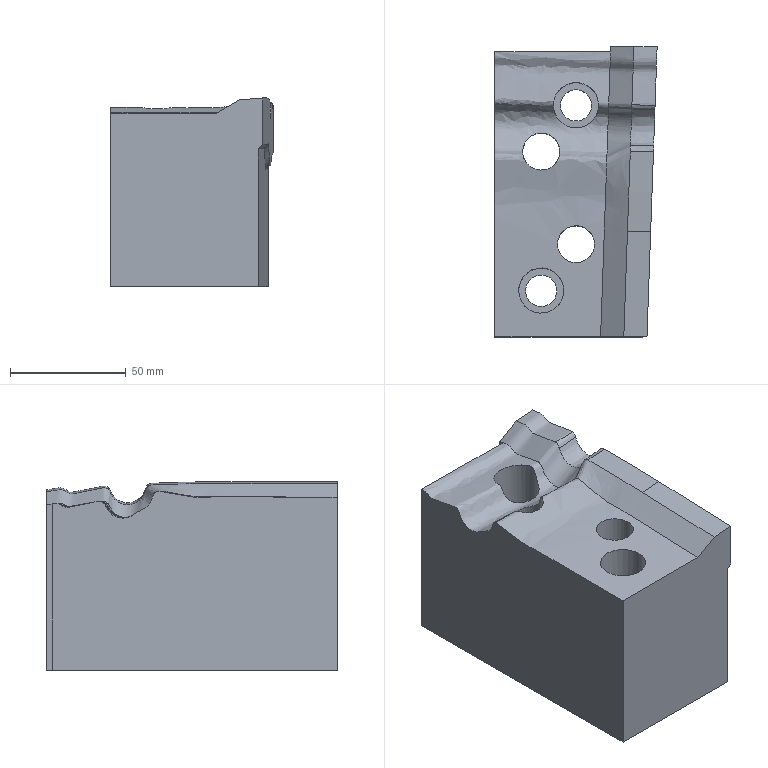Part | NX | features solid 2 | 1 solid | 26 faces | box 70 x 125.528 x 81.386 mm | volume 542744 mm3 | spline 11 | plane 9 | cylinder 6 | commonest cylinder face diameters 13.5 x2 16 x2 19.5 x2